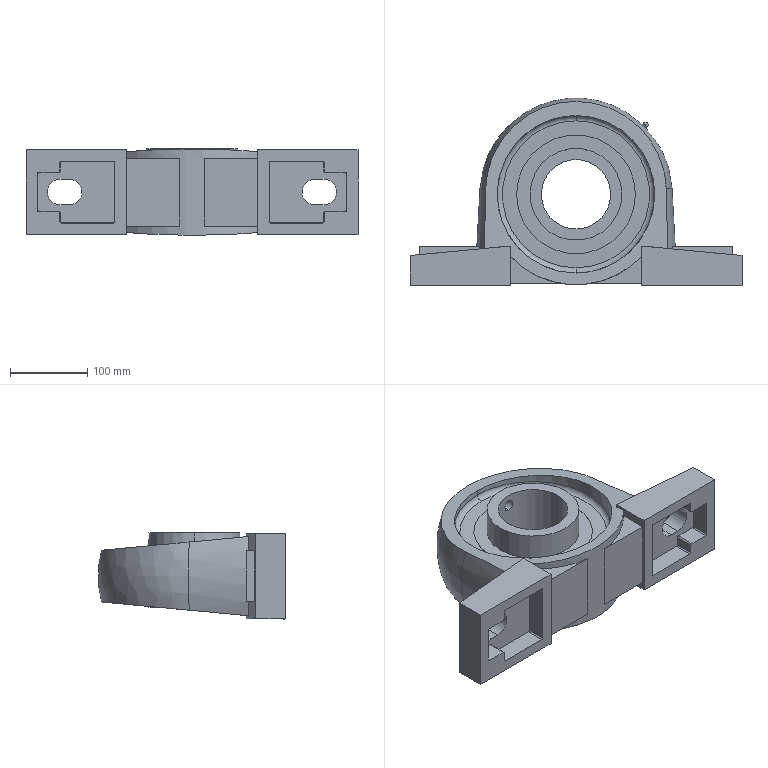Part | STEP file | GB/T7810-1995 pillow block bearing UCP318 | 1 solid | 123 faces | box 430 x 242.58 x 111.692 mm | volume 3436348 mm3 | plane 61 | cylinder 27 | cone 16 | sphere 8 | torus 6 | spline 3 | other 2 | commonest cylinder face diameters 119 x6 154.04 x6 204.086 x6 33 x4 14.701 x2 90 x2